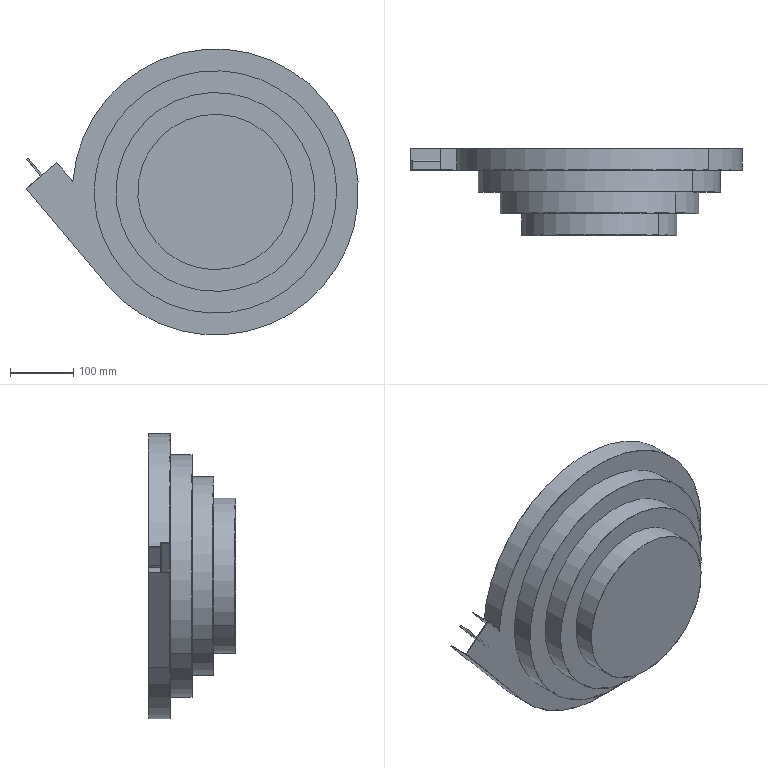Part | STEP file | 1 solid | 37 faces | box 524.053 x 137.2 x 450.8 mm | volume 389951 mm3 | plane 19 | cylinder 18 | commonest cylinder face diameters 2.94 x2 242.55 x2 245 x2 311.15 x2 313.6 x2 379.75 x2